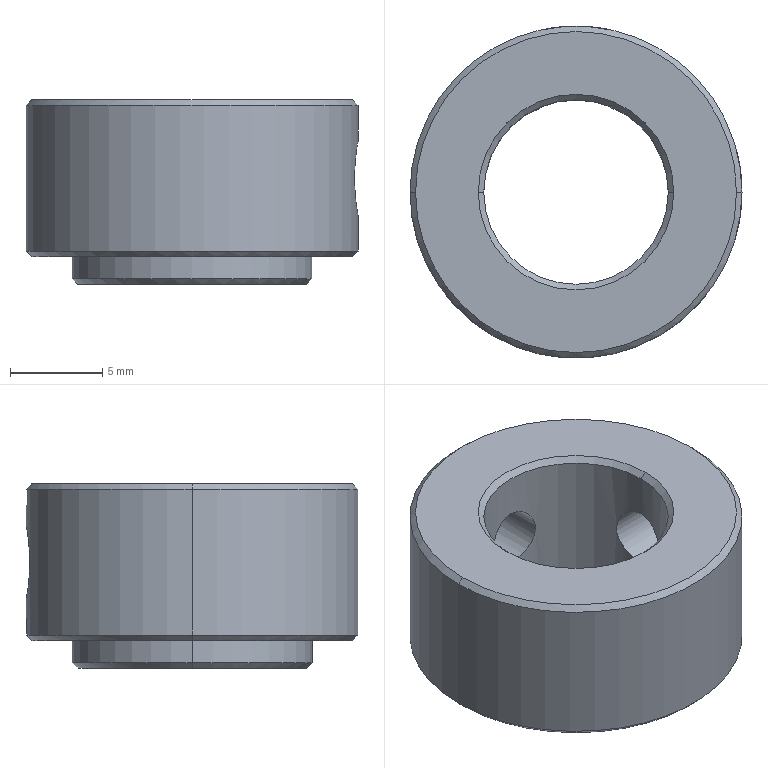Part | SolidWorks | features BaseBody 1 | 1 solid | 27 faces | box 18 x 18 x 10 mm | volume 1499 mm3 | cone 14 | cylinder 10 | plane 3 | commonest cylinder face diameters 3.242 x4 10 x2 13 x2 18 x2
STEP:
#1=CARTESIAN_POINT('',(0.,8.621,4.129));
#2=VERTEX_POINT('',#1);
#3=CARTESIAN_POINT('',(0.,9.,3.75));
#4=VERTEX_POINT('',#3);
#5=CARTESIAN_POINT('',(0.,9.003,3.747));
#6=DIRECTION('',(0.,0.7071,-0.7071));
#7=VECTOR('',#6,1000.);
#8=LINE('',#5,#7);
#9=EDGE_CURVE('',#2,#4,#8,.T.);
#10=ORIENTED_EDGE('',*,*,#9,.F.);
#11=CARTESIAN_POINT('',(0.,8.621,7.371));
#12=VERTEX_POINT('',#11);
#13=CARTESIAN_POINT('',(0.,8.621,5.75));
#14=DIRECTION('',(0.,-1.,0.));
#15=DIRECTION('',(0.,0.,1.));
#16=AXIS2_PLACEMENT_3D('',#13,#14,#15);
#17=CIRCLE('',#16,1.621);
#18=EDGE_CURVE('',#2,#12,#17,.T.);
#19=ORIENTED_EDGE('',*,*,#18,.T.);
#20=CARTESIAN_POINT('',(0.,9.,7.75));
#21=VERTEX_POINT('',#20);
#22=CARTESIAN_POINT('',(0.,9.003,7.753));
#23=DIRECTION('',(0.,0.7071,0.7071));
#24=VECTOR('',#23,1000.);
#25=LINE('',#22,#24);
#26=EDGE_CURVE('',#12,#21,#25,.T.);
#27=ORIENTED_EDGE('',*,*,#26,.T.);
#28=CARTESIAN_POINT('',(0.,9.,3.75));
#29=CARTESIAN_POINT('',(0.1256,9.,3.75));
#30=CARTESIAN_POINT('',(0.2518,8.997,3.765));
#31=CARTESIAN_POINT('',(0.4336,8.99,3.807));
#32=CARTESIAN_POINT('',(0.4933,8.987,3.825));
#33=CARTESIAN_POINT('',(0.6108,8.979,3.866));
#34=CARTESIAN_POINT('',(0.6697,8.975,3.891));
#35=CARTESIAN_POINT('',(0.8371,8.962,3.972));
#36=CARTESIAN_POINT('',(0.9418,8.951,4.036));
#37=CARTESIAN_POINT('',(1.089,8.934,4.15));
#38=CARTESIAN_POINT('',(1.136,8.928,4.19));
#39=CARTESIAN_POINT('',(1.227,8.916,4.277));
#40=CARTESIAN_POINT('',(1.272,8.91,4.324));
#41=CARTESIAN_POINT('',(1.394,8.892,4.465));
#42=CARTESIAN_POINT('',(1.466,8.88,4.566));
#43=CARTESIAN_POINT('',(1.591,8.859,4.78));
#44=CARTESIAN_POINT('',(1.644,8.849,4.895));
#45=CARTESIAN_POINT('',(1.772,8.824,5.25));
#46=CARTESIAN_POINT('',(1.815,8.815,5.495));
#47=CARTESIAN_POINT('',(1.815,8.815,5.875));
#48=CARTESIAN_POINT('',(1.805,8.817,6.));
#49=CARTESIAN_POINT('',(1.762,8.826,6.245));
#50=CARTESIAN_POINT('',(1.731,8.832,6.364));
#51=CARTESIAN_POINT('',(1.601,8.857,6.724));
#52=CARTESIAN_POINT('',(1.478,8.879,6.937));
#53=CARTESIAN_POINT('',(1.273,8.91,7.175));
#54=CARTESIAN_POINT('',(1.23,8.916,7.22));
#55=CARTESIAN_POINT('',(1.14,8.928,7.306));
#56=CARTESIAN_POINT('',(1.093,8.933,7.346));
#57=CARTESIAN_POINT('',(0.9931,8.945,7.424));
#58=CARTESIAN_POINT('',(0.9416,8.951,7.46));
#59=CARTESIAN_POINT('',(0.8357,8.961,7.525));
#60=CARTESIAN_POINT('',(0.7826,8.966,7.555));
#61=CARTESIAN_POINT('',(0.4976,8.989,7.692));
#62=CARTESIAN_POINT('',(0.2507,9.,7.75));
#63=CARTESIAN_POINT('',(0.,9.,7.75));
#64=B_SPLINE_CURVE_WITH_KNOTS('',3,(#28,#29,#30,#31,#32,#33,#34,#35,#36,#37,#38,#39,#40,#41,#42,#43,#44,#45,#46,#47,#48,#49,#50,#51,#52,#53,#54,#55,#56,#57,#58,#59,#60,#61,#62,#63),.UNSPECIFIED.,.F.,.F.,(4,2,2,2,2,2,2,2,2,2,2,2,2,2,2,2,2,4),(0.,0.0625,0.09375,0.125,0.1875,0.2187,0.25,0.3125,0.375,0.5,0.5625,0.625,0.75,0.7812,0.8125,0.8437,0.875,1.),.UNSPECIFIED.);
#65=EDGE_CURVE('',#4,#21,#64,.T.);
#66=ORIENTED_EDGE('',*,*,#65,.F.);
#67=EDGE_LOOP('',(#10,#19,#27,#66));
#68=FACE_OUTER_BOUND('',#67,.T.);
#69=CARTESIAN_POINT('',(0.,9.003,5.75));
#70=DIRECTION('',(0.,1.,0.));
#71=DIRECTION('',(0.,0.,1.));
#72=AXIS2_PLACEMENT_3D('',#69,#70,#71);
#73=CONICAL_SURFACE('',#72,2.003,0.7854);
#74=ADVANCED_FACE('',(#68),#73,.F.);
#75=CARTESIAN_POINT('',(8.621,0.,7.371));
#76=VERTEX_POINT('',#75);
#77=CARTESIAN_POINT('',(9.,0.,7.75));
#78=VERTEX_POINT('',#77);
#79=CARTESIAN_POINT('',(9.031,0.,7.781));
#80=DIRECTION('',(0.7071,0.,0.7071));
#81=VECTOR('',#80,1000.);
#82=LINE('',#79,#81);
#83=EDGE_CURVE('',#76,#78,#82,.T.);
#84=ORIENTED_EDGE('',*,*,#83,.F.);
#85=CARTESIAN_POINT('',(8.621,0.,4.129));
#86=VERTEX_POINT('',#85);
#87=CARTESIAN_POINT('',(8.621,0.,5.75));
#88=DIRECTION('',(-1.,0.,0.));
#89=DIRECTION('',(0.,0.,-1.));
#90=AXIS2_PLACEMENT_3D('',#87,#88,#89);
#91=CIRCLE('',#90,1.621);
#92=EDGE_CURVE('',#76,#86,#91,.T.);
#93=ORIENTED_EDGE('',*,*,#92,.T.);
#94=CARTESIAN_POINT('',(9.,0.,3.75));
#95=VERTEX_POINT('',#94);
#96=CARTESIAN_POINT('',(9.031,0.,3.719));
#97=DIRECTION('',(0.7071,0.,-0.7071));
#98=VECTOR('',#97,1000.);
#99=LINE('',#96,#98);
#100=EDGE_CURVE('',#86,#95,#99,.T.);
#101=ORIENTED_EDGE('',*,*,#100,.T.);
#102=CARTESIAN_POINT('',(9.,0.,7.75));
#103=CARTESIAN_POINT('',(9.,0.251,7.75));
#104=CARTESIAN_POINT('',(8.989,0.5004,7.691));
#105=CARTESIAN_POINT('',(8.962,0.8348,7.53));
#106=CARTESIAN_POINT('',(8.951,0.9395,7.465));
#107=CARTESIAN_POINT('',(8.934,1.086,7.352));
#108=CARTESIAN_POINT('',(8.928,1.133,7.312));
#109=CARTESIAN_POINT('',(8.916,1.224,7.226));
#110=CARTESIAN_POINT('',(8.91,1.27,7.178));
#111=CARTESIAN_POINT('',(8.892,1.392,7.038));
#112=CARTESIAN_POINT('',(8.88,1.464,6.937));
#113=CARTESIAN_POINT('',(8.859,1.589,6.724));
#114=CARTESIAN_POINT('',(8.849,1.642,6.609));
#115=CARTESIAN_POINT('',(8.833,1.728,6.373));
#116=CARTESIAN_POINT('',(8.826,1.76,6.253));
#117=CARTESIAN_POINT('',(8.817,1.804,6.008));
#118=CARTESIAN_POINT('',(8.815,1.815,5.883));
#119=CARTESIAN_POINT('',(8.815,1.815,5.632));
#120=CARTESIAN_POINT('',(8.817,1.805,5.506));
#121=CARTESIAN_POINT('',(8.826,1.762,5.257));
#122=CARTESIAN_POINT('',(8.832,1.731,5.136));
#123=CARTESIAN_POINT('',(8.848,1.646,4.9));
#124=CARTESIAN_POINT('',(8.858,1.594,4.788));
#125=CARTESIAN_POINT('',(8.874,1.499,4.624));
#126=CARTESIAN_POINT('',(8.88,1.466,4.571));
#127=CARTESIAN_POINT('',(8.892,1.394,4.47));
#128=CARTESIAN_POINT('',(8.897,1.356,4.422));
#129=CARTESIAN_POINT('',(8.916,1.232,4.278));
#130=CARTESIAN_POINT('',(8.928,1.144,4.193));
#131=CARTESIAN_POINT('',(8.945,0.9941,4.077));
#132=CARTESIAN_POINT('',(8.951,0.9428,4.041));
#133=CARTESIAN_POINT('',(8.961,0.837,3.975));
#134=CARTESIAN_POINT('',(8.966,0.7839,3.946));
#135=CARTESIAN_POINT('',(8.98,0.6128,3.863));
#136=CARTESIAN_POINT('',(8.987,0.4964,3.822));
#137=CARTESIAN_POINT('',(8.997,0.2502,3.764));
#138=CARTESIAN_POINT('',(9.,0.1257,3.75));
#139=CARTESIAN_POINT('',(9.,0.,3.75));
#140=B_SPLINE_CURVE_WITH_KNOTS('',3,(#102,#103,#104,#105,#106,#107,#108,#109,#110,#111,#112,#113,#114,#115,#116,#117,#118,#119,#120,#121,#122,#123,#124,#125,#126,#127,#128,#129,#130,#131,#132,#133,#134,#135,#136,#137,#138,#139),.UNSPECIFIED.,.F.,.F.,(4,2,2,2,2,2,2,2,2,2,2,2,2,2,2,2,2,2,4),(0.,0.125,0.1875,0.2187,0.25,0.3125,0.375,0.4375,0.5,0.5625,0.625,0.6875,0.7188,0.75,0.8125,0.8438,0.875,0.9375,1.),.UNSPECIFIED.);
#141=EDGE_CURVE('',#78,#95,#140,.T.);
#142=ORIENTED_EDGE('',*,*,#141,.F.);
#143=EDGE_LOOP('',(#84,#93,#101,#142));
#144=FACE_OUTER_BOUND('',#143,.T.);
#145=CARTESIAN_POINT('',(9.031,0.,5.75));
#146=DIRECTION('',(1.,0.,0.));
#147=DIRECTION('',(0.,0.,-1.));
#148=AXIS2_PLACEMENT_3D('',#145,#146,#147);
#149=CONICAL_SURFACE('',#148,2.031,0.7854);
#150=ADVANCED_FACE('',(#144),#149,.F.);
#151=CARTESIAN_POINT('',(5.,0.,0.3));
#152=VERTEX_POINT('',#151);
#153=CARTESIAN_POINT('',(5.3,0.,0.));
#154=VERTEX_POINT('',#153);
#155=CARTESIAN_POINT('',(5.3,0.,0.));
#156=DIRECTION('',(0.7071,0.,-0.7071));
#157=VECTOR('',#156,1000.);
#158=LINE('',#155,#157);
#159=EDGE_CURVE('',#152,#154,#158,.T.);
#160=ORIENTED_EDGE('',*,*,#159,.F.);
#161=CARTESIAN_POINT('',(-5.,0.,0.3));
#162=VERTEX_POINT('',#161);
#163=CARTESIAN_POINT('',(0.,0.,0.3));
#164=DIRECTION('',(0.,0.,1.));
#165=DIRECTION('',(-1.,0.,0.));
#166=AXIS2_PLACEMENT_3D('',#163,#164,#165);
#167=CIRCLE('',#166,5.);
#168=EDGE_CURVE('',#152,#162,#167,.T.);
#169=ORIENTED_EDGE('',*,*,#168,.T.);
#170=CARTESIAN_POINT('',(-5.3,0.,0.));
#171=VERTEX_POINT('',#170);
#172=CARTESIAN_POINT('',(-5.3,0.,0.));
#173=DIRECTION('',(-0.7071,0.,-0.7071));
#174=VECTOR('',#173,1000.);
#175=LINE('',#172,#174);
#176=EDGE_CURVE('',#162,#171,#175,.T.);
#177=ORIENTED_EDGE('',*,*,#176,.T.);
#178=CARTESIAN_POINT('',(0.,0.,0.));
#179=DIRECTION('',(0.,0.,1.));
#180=DIRECTION('',(-1.,0.,0.));
#181=AXIS2_PLACEMENT_3D('',#178,#179,#180);
#182=CIRCLE('',#181,5.3);
#183=EDGE_CURVE('',#154,#171,#182,.T.);
#184=ORIENTED_EDGE('',*,*,#183,.F.);
#185=EDGE_LOOP('',(#160,#169,#177,#184));
#186=FACE_OUTER_BOUND('',#185,.T.);
#187=CARTESIAN_POINT('',(0.,0.,0.));
#188=DIRECTION('',(0.,0.,-1.));
#189=DIRECTION('',(-1.,0.,0.));
#190=AXIS2_PLACEMENT_3D('',#187,#188,#189);
#191=CONICAL_SURFACE('',#190,5.3,0.7854);
#192=ADVANCED_FACE('',(#186),#191,.F.);
#193=CARTESIAN_POINT('',(0.,5.,4.129));
#194=VERTEX_POINT('',#193);
#195=CARTESIAN_POINT('',(0.,9.,4.129));
#196=DIRECTION('',(0.,1.,0.));
#197=VECTOR('',#196,1000.);
#198=LINE('',#195,#197);
#199=EDGE_CURVE('',#194,#2,#198,.T.);
#200=ORIENTED_EDGE('',*,*,#199,.F.);
#201=CARTESIAN_POINT('',(0.,5.,7.371));
#202=VERTEX_POINT('',#201);
#203=CARTESIAN_POINT('',(0.,5.,4.129));
#204=CARTESIAN_POINT('',(0.101,5.,4.129));
#205=CARTESIAN_POINT('',(0.2048,4.997,4.138));
#206=CARTESIAN_POINT('',(0.3616,4.987,4.169));
#207=CARTESIAN_POINT('',(0.414,4.983,4.182));
#208=CARTESIAN_POINT('',(0.4924,4.976,4.205));
#209=CARTESIAN_POINT('',(0.5316,4.972,4.218));
#210=CARTESIAN_POINT('',(0.577,4.967,4.235));
#211=CARTESIAN_POINT('',(0.5997,4.964,4.244));
#212=CARTESIAN_POINT('',(0.6094,4.963,4.248));
#213=CARTESIAN_POINT('',(0.6159,4.962,4.251));
#214=CARTESIAN_POINT('',(0.6202,4.961,4.252));
#215=CARTESIAN_POINT('',(0.6914,4.952,4.282));
#216=CARTESIAN_POINT('',(0.7729,4.94,4.321));
#217=CARTESIAN_POINT('',(0.9071,4.917,4.405));
#218=CARTESIAN_POINT('',(0.9537,4.908,4.438));
#219=CARTESIAN_POINT('',(1.025,4.894,4.494));
#220=CARTESIAN_POINT('',(1.049,4.889,4.514));
#221=CARTESIAN_POINT('',(1.097,4.878,4.556));
#222=CARTESIAN_POINT('',(1.12,4.873,4.578));
#223=CARTESIAN_POINT('',(1.247,4.843,4.704));
#224=CARTESIAN_POINT('',(1.321,4.823,4.805));
#225=CARTESIAN_POINT('',(1.405,4.799,4.939));
#226=CARTESIAN_POINT('',(1.428,4.792,4.982));
#227=CARTESIAN_POINT('',(1.457,4.783,5.04));
#228=CARTESIAN_POINT('',(1.466,4.78,5.059));
#229=CARTESIAN_POINT('',(1.479,4.776,5.085));
#230=CARTESIAN_POINT('',(1.484,4.775,5.098));
#231=CARTESIAN_POINT('',(1.491,4.773,5.113));
#232=CARTESIAN_POINT('',(1.493,4.772,5.119));
#233=CARTESIAN_POINT('',(1.495,4.771,5.123));
#234=CARTESIAN_POINT('',(1.495,4.771,5.124));
#235=CARTESIAN_POINT('',(1.583,4.744,5.336));
#236=CARTESIAN_POINT('',(1.621,4.73,5.551));
#237=CARTESIAN_POINT('',(1.621,4.73,5.851));
#238=CARTESIAN_POINT('',(1.612,4.733,5.954));
#239=CARTESIAN_POINT('',(1.581,4.744,6.111));
#240=CARTESIAN_POINT('',(1.568,4.748,6.163));
#241=CARTESIAN_POINT('',(1.545,4.755,6.242));
#242=CARTESIAN_POINT('',(1.532,4.76,6.282));
#243=CARTESIAN_POINT('',(1.515,4.765,6.327));
#244=CARTESIAN_POINT('',(1.506,4.768,6.35));
#245=CARTESIAN_POINT('',(1.502,4.769,6.36));
#246=CARTESIAN_POINT('',(1.499,4.77,6.367));
#247=CARTESIAN_POINT('',(1.497,4.771,6.371));
#248=CARTESIAN_POINT('',(1.47,4.779,6.437));
#249=CARTESIAN_POINT('',(1.433,4.791,6.516));
#250=CARTESIAN_POINT('',(1.349,4.815,6.65));
#251=CARTESIAN_POINT('',(1.317,4.824,6.697));
#252=CARTESIAN_POINT('',(1.26,4.839,6.771));
#253=CARTESIAN_POINT('',(1.239,4.844,6.796));
#254=CARTESIAN_POINT('',(1.195,4.855,6.846));
#255=CARTESIAN_POINT('',(1.171,4.861,6.872));
#256=CARTESIAN_POINT('',(1.05,4.89,6.993));
#257=CARTESIAN_POINT('',(0.9525,4.909,7.066));
#258=CARTESIAN_POINT('',(0.8184,4.932,7.15));
#259=CARTESIAN_POINT('',(0.7756,4.939,7.174));
#260=CARTESIAN_POINT('',(0.7153,4.948,7.205));
#261=CARTESIAN_POINT('',(0.6862,4.953,7.219));
#262=CARTESIAN_POINT('',(0.654,4.957,7.233));
#263=CARTESIAN_POINT('',(0.6385,4.959,7.24));
#264=CARTESIAN_POINT('',(0.6319,4.96,7.243));
#265=CARTESIAN_POINT('',(0.6275,4.96,7.245));
#266=CARTESIAN_POINT('',(0.6264,4.961,7.245));
#267=CARTESIAN_POINT('',(0.4163,4.987,7.333));
#268=CARTESIAN_POINT('',(0.2023,5.,7.371));
#269=CARTESIAN_POINT('',(0.,5.,7.371));
#270=B_SPLINE_CURVE_WITH_KNOTS('',3,(#203,#204,#205,#206,#207,#208,#209,#210,#211,#212,#213,#214,#215,#216,#217,#218,#219,#220,#221,#222,#223,#224,#225,#226,#227,#228,#229,#230,#231,#232,#233,#234,#235,#236,#237,#238,#239,#240,#241,#242,#243,#244,#245,#246,#247,#248,#249,#250,#251,#252,#253,#254,#255,#256,#257,#258,#259,#260,#261,#262,#263,#264,#265,#266,#267,#268,#269),.UNSPECIFIED.,.F.,.F.,(4,2,2,1,1,1,2,2,2,2,2,2,2,2,2,1,1,2,2,2,2,2,1,1,1,2,2,2,2,2,2,2,2,1,1,1,2,2,4),(0.,0.0625,0.09375,0.1094,0.1172,0.1211,0.123,0.125,0.1875,0.2187,0.2344,0.25,0.3125,0.3437,0.3594,0.3672,0.3711,0.373,0.375,0.5,0.5625,0.5938,0.6094,0.6172,0.6211,0.623,0.625,0.6875,0.7188,0.7344,0.75,0.8125,0.8438,0.8594,0.8672,0.8711,0.873,0.875,1.),.UNSPECIFIED.);
#271=EDGE_CURVE('',#194,#202,#270,.T.);
#272=ORIENTED_EDGE('',*,*,#271,.T.);
#273=CARTESIAN_POINT('',(0.,9.,7.371));
#274=DIRECTION('',(0.,1.,0.));
#275=VECTOR('',#274,1000.);
#276=LINE('',#273,#275);
#277=EDGE_CURVE('',#202,#12,#276,.T.);
#278=ORIENTED_EDGE('',*,*,#277,.T.);
#279=ORIENTED_EDGE('',*,*,#18,.F.);
#280=EDGE_LOOP('',(#200,#272,#278,#279));
#281=FACE_OUTER_BOUND('',#280,.T.);
#282=CARTESIAN_POINT('',(0.,9.,5.75));
#283=DIRECTION('',(0.,1.,0.));
#284=DIRECTION('',(0.,0.,1.));
#285=AXIS2_PLACEMENT_3D('',#282,#283,#284);
#286=CYLINDRICAL_SURFACE('',#285,1.621);
#287=ADVANCED_FACE('',(#281),#286,.F.);
#288=CARTESIAN_POINT('',(5.,0.,4.129));
#289=VERTEX_POINT('',#288);
#290=CARTESIAN_POINT('',(0.,0.,4.129));
#291=DIRECTION('',(-1.,0.,0.));
#292=VECTOR('',#291,1000.);
#293=LINE('',#290,#292);
#294=EDGE_CURVE('',#86,#289,#293,.T.);
#295=ORIENTED_EDGE('',*,*,#294,.F.);
#296=ORIENTED_EDGE('',*,*,#92,.F.);
#297=CARTESIAN_POINT('',(5.,0.,7.371));
#298=VERTEX_POINT('',#297);
#299=CARTESIAN_POINT('',(0.,0.,7.371));
#300=DIRECTION('',(-1.,0.,0.));
#301=VECTOR('',#300,1000.);
#302=LINE('',#299,#301);
#303=EDGE_CURVE('',#76,#298,#302,.T.);
#304=ORIENTED_EDGE('',*,*,#303,.T.);
#305=CARTESIAN_POINT('',(5.,0.,7.371));
#306=CARTESIAN_POINT('',(5.,0.1011,7.371));
#307=CARTESIAN_POINT('',(4.997,0.205,7.362));
#308=CARTESIAN_POINT('',(4.987,0.362,7.331));
#309=CARTESIAN_POINT('',(4.983,0.4145,7.318));
#310=CARTESIAN_POINT('',(4.976,0.493,7.294));
#311=CARTESIAN_POINT('',(4.972,0.5322,7.282));
#312=CARTESIAN_POINT('',(4.967,0.5778,7.265));
#313=CARTESIAN_POINT('',(4.964,0.6005,7.256));
#314=CARTESIAN_POINT('',(4.963,0.6102,7.252));
#315=CARTESIAN_POINT('',(4.962,0.6167,7.249));
#316=CARTESIAN_POINT('',(4.961,0.621,7.247));
#317=CARTESIAN_POINT('',(4.952,0.6921,7.218));
#318=CARTESIAN_POINT('',(4.94,0.7736,7.178));
#319=CARTESIAN_POINT('',(4.917,0.9077,7.094));
#320=CARTESIAN_POINT('',(4.908,0.9543,7.062));
#321=CARTESIAN_POINT('',(4.893,1.026,7.006));
#322=CARTESIAN_POINT('',(4.888,1.05,6.986));
#323=CARTESIAN_POINT('',(4.881,1.086,6.954));
#324=CARTESIAN_POINT('',(4.878,1.098,6.943));
#325=CARTESIAN_POINT('',(4.872,1.122,6.92));
#326=CARTESIAN_POINT('',(4.87,1.133,6.909));
#327=CARTESIAN_POINT('',(4.855,1.198,6.845));
#328=CARTESIAN_POINT('',(4.844,1.239,6.797));
#329=CARTESIAN_POINT('',(4.831,1.288,6.735));
#330=CARTESIAN_POINT('',(4.828,1.302,6.716));
#331=CARTESIAN_POINT('',(4.822,1.321,6.69));
#332=CARTESIAN_POINT('',(4.82,1.329,6.678));
#333=CARTESIAN_POINT('',(4.818,1.338,6.665));
#334=CARTESIAN_POINT('',(4.817,1.342,6.66));
#335=CARTESIAN_POINT('',(4.816,1.344,6.656));
#336=CARTESIAN_POINT('',(4.816,1.344,6.656));
#337=CARTESIAN_POINT('',(4.806,1.379,6.604));
#338=CARTESIAN_POINT('',(4.798,1.408,6.556));
#339=CARTESIAN_POINT('',(4.787,1.445,6.486));
#340=CARTESIAN_POINT('',(4.782,1.462,6.451));
#341=CARTESIAN_POINT('',(4.776,1.48,6.412));
#342=CARTESIAN_POINT('',(4.774,1.487,6.395));
#343=CARTESIAN_POINT('',(4.772,1.492,6.384));
#344=CARTESIAN_POINT('',(4.772,1.494,6.379));
#345=CARTESIAN_POINT('',(4.744,1.583,6.165));
#346=CARTESIAN_POINT('',(4.73,1.621,5.951));
#347=CARTESIAN_POINT('',(4.73,1.621,5.65));
#348=CARTESIAN_POINT('',(4.733,1.612,5.547));
#349=CARTESIAN_POINT('',(4.743,1.581,5.39));
#350=CARTESIAN_POINT('',(4.748,1.569,5.338));
#351=CARTESIAN_POINT('',(4.755,1.545,5.259));
#352=CARTESIAN_POINT('',(4.76,1.532,5.22));
#353=CARTESIAN_POINT('',(4.765,1.515,5.174));
#354=CARTESIAN_POINT('',(4.767,1.508,5.154));
#355=CARTESIAN_POINT('',(4.769,1.502,5.141));
#356=CARTESIAN_POINT('',(4.77,1.499,5.134));
#357=CARTESIAN_POINT('',(4.776,1.479,5.084));
#358=CARTESIAN_POINT('',(4.783,1.458,5.039));
#359=CARTESIAN_POINT('',(4.794,1.421,4.969));
#360=CARTESIAN_POINT('',(4.8,1.401,4.933));
#361=CARTESIAN_POINT('',(4.807,1.375,4.891));
#362=CARTESIAN_POINT('',(4.811,1.361,4.87));
#363=CARTESIAN_POINT('',(4.813,1.355,4.861));
#364=CARTESIAN_POINT('',(4.814,1.351,4.854));
#365=CARTESIAN_POINT('',(4.815,1.348,4.85));
#366=CARTESIAN_POINT('',(4.82,1.329,4.821));
#367=CARTESIAN_POINT('',(4.827,1.305,4.787));
#368=CARTESIAN_POINT('',(4.84,1.256,4.725));
#369=CARTESIAN_POINT('',(4.845,1.237,4.702));
#370=CARTESIAN_POINT('',(4.852,1.206,4.667));
#371=CARTESIAN_POINT('',(4.855,1.195,4.655));
#372=CARTESIAN_POINT('',(4.861,1.172,4.63));
#373=CARTESIAN_POINT('',(4.864,1.159,4.617));
#374=CARTESIAN_POINT('',(4.889,1.05,4.508));
#375=CARTESIAN_POINT('',(4.909,0.9526,4.434));
#376=CARTESIAN_POINT('',(4.932,0.8183,4.35));
#377=CARTESIAN_POINT('',(4.939,0.7755,4.326));
#378=CARTESIAN_POINT('',(4.948,0.7151,4.295));
#379=CARTESIAN_POINT('',(4.953,0.6859,4.281));
#380=CARTESIAN_POINT('',(4.957,0.6538,4.267));
#381=CARTESIAN_POINT('',(4.959,0.6382,4.26));
#382=CARTESIAN_POINT('',(4.96,0.6316,4.257));
#383=CARTESIAN_POINT('',(4.96,0.6272,4.255));
#384=CARTESIAN_POINT('',(4.961,0.6262,4.255));
#385=CARTESIAN_POINT('',(4.987,0.4161,4.167));
#386=CARTESIAN_POINT('',(5.,0.2022,4.129));
#387=CARTESIAN_POINT('',(5.,0.,4.129));
#388=B_SPLINE_CURVE_WITH_KNOTS('',3,(#305,#306,#307,#308,#309,#310,#311,#312,#313,#314,#315,#316,#317,#318,#319,#320,#321,#322,#323,#324,#325,#326,#327,#328,#329,#330,#331,#332,#333,#334,#335,#336,#337,#338,#339,#340,#341,#342,#343,#344,#345,#346,#347,#348,#349,#350,#351,#352,#353,#354,#355,#356,#357,#358,#359,#360,#361,#362,#363,#364,#365,#366,#367,#368,#369,#370,#371,#372,#373,#374,#375,#376,#377,#378,#379,#380,#381,#382,#383,#384,#385,#386,#387),.UNSPECIFIED.,.F.,.F.,(4,2,2,1,1,1,2,2,2,2,2,2,2,2,2,1,1,2,2,2,1,1,2,2,2,2,2,1,1,2,2,2,1,1,1,2,2,2,2,2,2,2,2,1,1,1,2,2,4),(0.,0.0625,0.09375,0.1094,0.1172,0.1211,0.123,0.125,0.1875,0.2188,0.2344,0.2422,0.25,0.2813,0.2969,0.3047,0.3086,0.3105,0.3125,0.3438,0.3594,0.3672,0.3711,0.375,0.5,0.5625,0.5938,0.6094,0.6172,0.6211,0.625,0.6563,0.6719,0.6797,0.6836,0.6855,0.6875,0.7188,0.7344,0.7422,0.75,0.8125,0.8438,0.8594,0.8672,0.8711,0.873,0.875,1.),.UNSPECIFIED.);
#389=EDGE_CURVE('',#298,#289,#388,.T.);
#390=ORIENTED_EDGE('',*,*,#389,.T.);
#391=EDGE_LOOP('',(#295,#296,#304,#390));
#392=FACE_OUTER_BOUND('',#391,.T.);
#393=CARTESIAN_POINT('',(0.,0.,5.75));
#394=DIRECTION('',(-1.,0.,0.));
#395=DIRECTION('',(0.,0.,1.));
#396=AXIS2_PLACEMENT_3D('',#393,#394,#395);
#397=CYLINDRICAL_SURFACE('',#396,1.621);
#398=ADVANCED_FACE('',(#392),#397,.F.);
#399=CARTESIAN_POINT('',(0.,0.,0.));
#400=DIRECTION('',(0.,0.,1.));
#401=DIRECTION('',(-1.,0.,0.));
#402=AXIS2_PLACEMENT_3D('',#399,#400,#401);
#403=CIRCLE('',#402,5.3);
#404=EDGE_CURVE('',#171,#154,#403,.T.);
#405=ORIENTED_EDGE('',*,*,#404,.T.);
#406=ORIENTED_EDGE('',*,*,#183,.T.);
#407=EDGE_LOOP('',(#405,#406));
#408=FACE_BOUND('',#407,.T.);
#409=CARTESIAN_POINT('',(6.2,0.,0.));
#410=VERTEX_POINT('',#409);
#411=CARTESIAN_POINT('',(-6.2,0.,0.));
#412=VERTEX_POINT('',#411);
#413=CARTESIAN_POINT('',(0.,0.,0.));
#414=DIRECTION('',(0.,0.,1.));
#415=DIRECTION('',(1.,0.,0.));
#416=AXIS2_PLACEMENT_3D('',#413,#414,#415);
#417=CIRCLE('',#416,6.2);
#418=EDGE_CURVE('',#410,#412,#417,.T.);
#419=ORIENTED_EDGE('',*,*,#418,.F.);
#420=CARTESIAN_POINT('',(0.,0.,0.));
#421=DIRECTION('',(0.,0.,1.));
#422=DIRECTION('',(1.,0.,0.));
#423=AXIS2_PLACEMENT_3D('',#420,#421,#422);
#424=CIRCLE('',#423,6.2);
#425=EDGE_CURVE('',#412,#410,#424,.T.);
#426=ORIENTED_EDGE('',*,*,#425,.F.);
#427=EDGE_LOOP('',(#419,#426));
#428=FACE_OUTER_BOUND('',#427,.T.);
#429=CARTESIAN_POINT('',(0.,5.3,0.));
#430=DIRECTION('',(0.,0.,-1.));
#431=DIRECTION('',(0.,-1.,0.));
#432=AXIS2_PLACEMENT_3D('',#429,#430,#431);
#433=PLANE('',#432);
#434=ADVANCED_FACE('',(#408,#428),#433,.T.);
#435=CARTESIAN_POINT('',(0.,5.,7.371));
#436=CARTESIAN_POINT('',(-0.1011,5.,7.371));
#437=CARTESIAN_POINT('',(-0.205,4.997,7.362));
#438=CARTESIAN_POINT('',(-0.362,4.987,7.331));
#439=CARTESIAN_POINT('',(-0.4145,4.983,7.318));
#440=CARTESIAN_POINT('',(-0.493,4.976,7.294));
#441=CARTESIAN_POINT('',(-0.5322,4.972,7.282));
#442=CARTESIAN_POINT('',(-0.5778,4.967,7.265));
#443=CARTESIAN_POINT('',(-0.6005,4.964,7.256));
#444=CARTESIAN_POINT('',(-0.6102,4.963,7.252));
#445=CARTESIAN_POINT('',(-0.6167,4.962,7.249));
#446=CARTESIAN_POINT('',(-0.621,4.961,7.247));
#447=CARTESIAN_POINT('',(-0.6921,4.952,7.218));
#448=CARTESIAN_POINT('',(-0.7736,4.94,7.178));
#449=CARTESIAN_POINT('',(-0.9077,4.917,7.094));
#450=CARTESIAN_POINT('',(-0.9543,4.908,7.062));
#451=CARTESIAN_POINT('',(-1.026,4.893,7.006));
#452=CARTESIAN_POINT('',(-1.05,4.888,6.986));
#453=CARTESIAN_POINT('',(-1.086,4.881,6.954));
#454=CARTESIAN_POINT('',(-1.098,4.878,6.943));
#455=CARTESIAN_POINT('',(-1.122,4.872,6.92));
#456=CARTESIAN_POINT('',(-1.133,4.87,6.909));
#457=CARTESIAN_POINT('',(-1.198,4.855,6.845));
#458=CARTESIAN_POINT('',(-1.239,4.844,6.797));
#459=CARTESIAN_POINT('',(-1.288,4.831,6.735));
#460=CARTESIAN_POINT('',(-1.302,4.828,6.716));
#461=CARTESIAN_POINT('',(-1.321,4.822,6.69));
#462=CARTESIAN_POINT('',(-1.329,4.82,6.678));
#463=CARTESIAN_POINT('',(-1.338,4.818,6.665));
#464=CARTESIAN_POINT('',(-1.342,4.817,6.66));
#465=CARTESIAN_POINT('',(-1.344,4.816,6.656));
#466=CARTESIAN_POINT('',(-1.344,4.816,6.656));
#467=CARTESIAN_POINT('',(-1.379,4.806,6.604));
#468=CARTESIAN_POINT('',(-1.408,4.798,6.556));
#469=CARTESIAN_POINT('',(-1.445,4.787,6.486));
#470=CARTESIAN_POINT('',(-1.462,4.782,6.451));
#471=CARTESIAN_POINT('',(-1.48,4.776,6.412));
#472=CARTESIAN_POINT('',(-1.487,4.774,6.395));
#473=CARTESIAN_POINT('',(-1.492,4.772,6.384));
#474=CARTESIAN_POINT('',(-1.494,4.772,6.379));
#475=CARTESIAN_POINT('',(-1.583,4.744,6.165));
#476=CARTESIAN_POINT('',(-1.621,4.73,5.951));
#477=CARTESIAN_POINT('',(-1.621,4.73,5.65));
#478=CARTESIAN_POINT('',(-1.612,4.733,5.547));
#479=CARTESIAN_POINT('',(-1.581,4.743,5.39));
#480=CARTESIAN_POINT('',(-1.569,4.748,5.338));
#481=CARTESIAN_POINT('',(-1.545,4.755,5.259));
#482=CARTESIAN_POINT('',(-1.532,4.76,5.22));
#483=CARTESIAN_POINT('',(-1.515,4.765,5.174));
#484=CARTESIAN_POINT('',(-1.508,4.767,5.154));
#485=CARTESIAN_POINT('',(-1.502,4.769,5.141));
#486=CARTESIAN_POINT('',(-1.499,4.77,5.134));
#487=CARTESIAN_POINT('',(-1.479,4.776,5.084));
#488=CARTESIAN_POINT('',(-1.458,4.783,5.039));
#489=CARTESIAN_POINT('',(-1.421,4.794,4.969));
#490=CARTESIAN_POINT('',(-1.401,4.8,4.933));
#491=CARTESIAN_POINT('',(-1.375,4.807,4.891));
#492=CARTESIAN_POINT('',(-1.361,4.811,4.87));
#493=CARTESIAN_POINT('',(-1.355,4.813,4.861));
#494=CARTESIAN_POINT('',(-1.351,4.814,4.854));
#495=CARTESIAN_POINT('',(-1.348,4.815,4.85));
#496=CARTESIAN_POINT('',(-1.329,4.82,4.821));
#497=CARTESIAN_POINT('',(-1.305,4.827,4.787));
#498=CARTESIAN_POINT('',(-1.256,4.84,4.725));
#499=CARTESIAN_POINT('',(-1.237,4.845,4.702));
#500=CARTESIAN_POINT('',(-1.206,4.852,4.667));
#501=CARTESIAN_POINT('',(-1.195,4.855,4.655));
#502=CARTESIAN_POINT('',(-1.172,4.861,4.63));
#503=CARTESIAN_POINT('',(-1.159,4.864,4.617));
#504=CARTESIAN_POINT('',(-1.05,4.889,4.508));
#505=CARTESIAN_POINT('',(-0.9526,4.909,4.434));
#506=CARTESIAN_POINT('',(-0.8183,4.932,4.35));
#507=CARTESIAN_POINT('',(-0.7755,4.939,4.326));
#508=CARTESIAN_POINT('',(-0.7151,4.948,4.295));
#509=CARTESIAN_POINT('',(-0.6859,4.953,4.281));
#510=CARTESIAN_POINT('',(-0.6538,4.957,4.267));
#511=CARTESIAN_POINT('',(-0.6382,4.959,4.26));
#512=CARTESIAN_POINT('',(-0.6316,4.96,4.257));
#513=CARTESIAN_POINT('',(-0.6272,4.96,4.255));
#514=CARTESIAN_POINT('',(-0.6262,4.961,4.255));
#515=CARTESIAN_POINT('',(-0.4161,4.987,4.167));
#516=CARTESIAN_POINT('',(-0.2022,5.,4.129));
#517=CARTESIAN_POINT('',(0.,5.,4.129));
#518=B_SPLINE_CURVE_WITH_KNOTS('',3,(#435,#436,#437,#438,#439,#440,#441,#442,#443,#444,#445,#446,#447,#448,#449,#450,#451,#452,#453,#454,#455,#456,#457,#458,#459,#460,#461,#462,#463,#464,#465,#466,#467,#468,#469,#470,#471,#472,#473,#474,#475,#476,#477,#478,#479,#480,#481,#482,#483,#484,#485,#486,#487,#488,#489,#490,#491,#492,#493,#494,#495,#496,#497,#498,#499,#500,#501,#502,#503,#504,#505,#506,#507,#508,#509,#510,#511,#512,#513,#514,#515,#516,#517),.UNSPECIFIED.,.F.,.F.,(4,2,2,1,1,1,2,2,2,2,2,2,2,2,2,1,1,2,2,2,1,1,2,2,2,2,2,1,1,2,2,2,1,1,1,2,2,2,2,2,2,2,2,1,1,1,2,2,4),(0.,0.0625,0.09375,0.1094,0.1172,0.1211,0.123,0.125,0.1875,0.2188,0.2344,0.2422,0.25,0.2813,0.2969,0.3047,0.3086,0.3105,0.3125,0.3438,0.3594,0.3672,0.3711,0.375,0.5,0.5625,0.5938,0.6094,0.6172,0.6211,0.625,0.6563,0.6719,0.6797,0.6836,0.6855,0.6875,0.7188,0.7344,0.7422,0.75,0.8125,0.8438,0.8594,0.8672,0.8711,0.873,0.875,1.),.UNSPECIFIED.);
#519=EDGE_CURVE('',#202,#194,#518,.T.);
#520=ORIENTED_EDGE('',*,*,#519,.F.);
#521=ORIENTED_EDGE('',*,*,#271,.F.);
#522=EDGE_LOOP('',(#520,#521));
#523=FACE_BOUND('',#522,.T.);
#524=CARTESIAN_POINT('',(5.,0.,9.7));
#525=VERTEX_POINT('',#524);
#526=CARTESIAN_POINT('',(5.,0.,0.));
#527=DIRECTION('',(0.,0.,-1.));
#528=VECTOR('',#527,1000.);
#529=LINE('',#526,#528);
#530=EDGE_CURVE('',#525,#298,#529,.T.);
#531=ORIENTED_EDGE('',*,*,#530,.F.);
#532=CARTESIAN_POINT('',(-5.,0.,9.7));
#533=VERTEX_POINT('',#532);
#534=CARTESIAN_POINT('',(0.,0.,9.7));
#535=DIRECTION('',(0.,0.,1.));
#536=DIRECTION('',(-1.,0.,0.));
#537=AXIS2_PLACEMENT_3D('',#534,#535,#536);
#538=CIRCLE('',#537,5.);
#539=EDGE_CURVE('',#525,#533,#538,.T.);
#540=ORIENTED_EDGE('',*,*,#539,.T.);
#541=CARTESIAN_POINT('',(-5.,0.,0.));
#542=DIRECTION('',(0.,0.,-1.));
#543=VECTOR('',#542,1000.);
#544=LINE('',#541,#543);
#545=EDGE_CURVE('',#533,#162,#544,.T.);
#546=ORIENTED_EDGE('',*,*,#545,.T.);
#547=ORIENTED_EDGE('',*,*,#168,.F.);
#548=CARTESIAN_POINT('',(5.,0.,0.));
#549=DIRECTION('',(0.,0.,-1.));
#550=VECTOR('',#549,1000.);
#551=LINE('',#548,#550);
#552=EDGE_CURVE('',#289,#152,#551,.T.);
#553=ORIENTED_EDGE('',*,*,#552,.F.);
#554=ORIENTED_EDGE('',*,*,#389,.F.);
#555=EDGE_LOOP('',(#531,#540,#546,#547,#553,#554));
#556=FACE_OUTER_BOUND('',#555,.T.);
#557=CARTESIAN_POINT('',(0.,0.,0.));
#558=DIRECTION('',(0.,0.,-1.));
#559=DIRECTION('',(-1.,0.,0.));
#560=AXIS2_PLACEMENT_3D('',#557,#558,#559);
#561=CYLINDRICAL_SURFACE('',#560,5.);
#562=ADVANCED_FACE('',(#523,#556),#561,.F.);
#563=CARTESIAN_POINT('',(-6.5,0.,0.3));
#564=VERTEX_POINT('',#563);
#565=CARTESIAN_POINT('',(-6.5,0.,0.3));
#566=DIRECTION('',(-0.7071,0.,0.7071));
#567=VECTOR('',#566,1000.);
#568=LINE('',#565,#567);
#569=EDGE_CURVE('',#412,#564,#568,.T.);
#570=ORIENTED_EDGE('',*,*,#569,.F.);
#571=ORIENTED_EDGE('',*,*,#425,.T.);
#572=CARTESIAN_POINT('',(6.5,0.,0.3));
#573=VERTEX_POINT('',#572);
#574=CARTESIAN_POINT('',(6.5,0.,0.3));
#575=DIRECTION('',(0.7071,0.,0.7071));
#576=VECTOR('',#575,1000.);
#577=LINE('',#574,#576);
#578=EDGE_CURVE('',#410,#573,#577,.T.);
#579=ORIENTED_EDGE('',*,*,#578,.T.);
#580=CARTESIAN_POINT('',(0.,0.,0.3));
#581=DIRECTION('',(0.,0.,1.));
#582=DIRECTION('',(-1.,0.,0.));
#583=AXIS2_PLACEMENT_3D('',#580,#581,#582);
#584=CIRCLE('',#583,6.5);
#585=EDGE_CURVE('',#564,#573,#584,.T.);
#586=ORIENTED_EDGE('',*,*,#585,.F.);
#587=EDGE_LOOP('',(#570,#571,#579,#586));
#588=FACE_OUTER_BOUND('',#587,.T.);
#589=CARTESIAN_POINT('',(0.,0.,0.3));
#590=DIRECTION('',(0.,0.,1.));
#591=DIRECTION('',(1.,0.,0.));
#592=AXIS2_PLACEMENT_3D('',#589,#590,#591);
#593=CONICAL_SURFACE('',#592,6.5,0.7854);
#594=ADVANCED_FACE('',(#588),#593,.T.);
#595=CARTESIAN_POINT('',(-5.3,0.,10.));
#596=VERTEX_POINT('',#595);
#597=CARTESIAN_POINT('',(-5.3,0.,10.));
#598=DIRECTION('',(-0.7071,0.,0.7071));
#599=VECTOR('',#598,1000.);
#600=LINE('',#597,#599);
#601=EDGE_CURVE('',#533,#596,#600,.T.);
#602=ORIENTED_EDGE('',*,*,#601,.F.);
#603=ORIENTED_EDGE('',*,*,#539,.F.);
#604=CARTESIAN_POINT('',(5.3,0.,10.));
#605=VERTEX_POINT('',#604);
#606=CARTESIAN_POINT('',(5.3,0.,10.));
#607=DIRECTION('',(0.7071,0.,0.7071));
#608=VECTOR('',#607,1000.);
#609=LINE('',#606,#608);
#610=EDGE_CURVE('',#525,#605,#609,.T.);
#611=ORIENTED_EDGE('',*,*,#610,.T.);
#612=CARTESIAN_POINT('',(0.,0.,10.));
#613=DIRECTION('',(0.,0.,-1.));
#614=DIRECTION('',(1.,0.,0.));
#615=AXIS2_PLACEMENT_3D('',#612,#613,#614);
#616=CIRCLE('',#615,5.3);
#617=EDGE_CURVE('',#596,#605,#616,.T.);
#618=ORIENTED_EDGE('',*,*,#617,.F.);
#619=EDGE_LOOP('',(#602,#603,#611,#618));
#620=FACE_OUTER_BOUND('',#619,.T.);
#621=CARTESIAN_POINT('',(0.,0.,10.));
#622=DIRECTION('',(0.,0.,1.));
#623=DIRECTION('',(1.,0.,0.));
#624=AXIS2_PLACEMENT_3D('',#621,#622,#623);
#625=CONICAL_SURFACE('',#624,5.3,0.7854);
#626=ADVANCED_FACE('',(#620),#625,.F.);
#627=CARTESIAN_POINT('',(6.5,0.,1.5));
#628=VERTEX_POINT('',#627);
#629=CARTESIAN_POINT('',(6.5,0.,0.));
#630=DIRECTION('',(0.,0.,-1.));
#631=VECTOR('',#630,1000.);
#632=LINE('',#629,#631);
#633=EDGE_CURVE('',#628,#573,#632,.T.);
#634=ORIENTED_EDGE('',*,*,#633,.F.);
#635=CARTESIAN_POINT('',(-6.5,0.,1.5));
#636=VERTEX_POINT('',#635);
#637=CARTESIAN_POINT('',(0.,0.,1.5));
#638=DIRECTION('',(0.,0.,1.));
#639=DIRECTION('',(-1.,0.,0.));
#640=AXIS2_PLACEMENT_3D('',#637,#638,#639);
#641=CIRCLE('',#640,6.5);
#642=EDGE_CURVE('',#636,#628,#641,.T.);
#643=ORIENTED_EDGE('',*,*,#642,.F.);
#644=CARTESIAN_POINT('',(-6.5,0.,0.));
#645=DIRECTION('',(0.,0.,-1.));
#646=VECTOR('',#645,1000.);
#647=LINE('',#644,#646);
#648=EDGE_CURVE('',#636,#564,#647,.T.);
#649=ORIENTED_EDGE('',*,*,#648,.T.);
#650=ORIENTED_EDGE('',*,*,#585,.T.);
#651=EDGE_LOOP('',(#634,#643,#649,#650));
#652=FACE_OUTER_BOUND('',#651,.T.);
#653=CARTESIAN_POINT('',(0.,0.,0.));
#654=DIRECTION('',(0.,0.,-1.));
#655=DIRECTION('',(-1.,0.,0.));
#656=AXIS2_PLACEMENT_3D('',#653,#654,#655);
#657=CYLINDRICAL_SURFACE('',#656,6.5);
#658=ADVANCED_FACE('',(#652),#657,.T.);
#659=CARTESIAN_POINT('',(0.,0.,10.));
#660=DIRECTION('',(0.,0.,-1.));
#661=DIRECTION('',(1.,0.,0.));
#662=AXIS2_PLACEMENT_3D('',#659,#660,#661);
#663=CIRCLE('',#662,5.3);
#664=EDGE_CURVE('',#605,#596,#663,.T.);
#665=ORIENTED_EDGE('',*,*,#664,.T.);
#666=ORIENTED_EDGE('',*,*,#617,.T.);
#667=EDGE_LOOP('',(#665,#666));
#668=FACE_BOUND('',#667,.T.);
#669=CARTESIAN_POINT('',(-8.7,0.,10.));
#670=VERTEX_POINT('',#669);
#671=CARTESIAN_POINT('',(8.7,0.,10.));
#672=VERTEX_POINT('',#671);
#673=CARTESIAN_POINT('',(0.,0.,10.));
#674=DIRECTION('',(0.,0.,-1.));
#675=DIRECTION('',(-1.,0.,0.));
#676=AXIS2_PLACEMENT_3D('',#673,#674,#675);
#677=CIRCLE('',#676,8.7);
#678=EDGE_CURVE('',#670,#672,#677,.T.);
#679=ORIENTED_EDGE('',*,*,#678,.F.);
#680=CARTESIAN_POINT('',(0.,0.,10.));
#681=DIRECTION('',(0.,0.,-1.));
#682=DIRECTION('',(-1.,0.,0.));
#683=AXIS2_PLACEMENT_3D('',#680,#681,#682);
#684=CIRCLE('',#683,8.7);
#685=EDGE_CURVE('',#672,#670,#684,.T.);
#686=ORIENTED_EDGE('',*,*,#685,.F.);
#687=EDGE_LOOP('',(#679,#686));
#688=FACE_OUTER_BOUND('',#687,.T.);
#689=CARTESIAN_POINT('',(0.,8.7,10.));
#690=DIRECTION('',(0.,0.,1.));
#691=DIRECTION('',(1.,0.,0.));
#692=AXIS2_PLACEMENT_3D('',#689,#690,#691);
#693=PLANE('',#692);
#694=ADVANCED_FACE('',(#668,#688),#693,.T.);
#695=ORIENTED_EDGE('',*,*,#642,.T.);
#696=CARTESIAN_POINT('',(0.,0.,1.5));
#697=DIRECTION('',(0.,0.,1.));
#698=DIRECTION('',(-1.,0.,0.));
#699=AXIS2_PLACEMENT_3D('',#696,#697,#698);
#700=CIRCLE('',#699,6.5);
#701=EDGE_CURVE('',#628,#636,#700,.T.);
#702=ORIENTED_EDGE('',*,*,#701,.T.);
#703=EDGE_LOOP('',(#695,#702));
#704=FACE_BOUND('',#703,.T.);
#705=CARTESIAN_POINT('',(8.7,0.,1.5));
#706=VERTEX_POINT('',#705);
#707=CARTESIAN_POINT('',(-8.7,0.,1.5));
#708=VERTEX_POINT('',#707);
#709=CARTESIAN_POINT('',(0.,0.,1.5));
#710=DIRECTION('',(0.,0.,1.));
#711=DIRECTION('',(1.,0.,0.));
#712=AXIS2_PLACEMENT_3D('',#709,#710,#711);
#713=CIRCLE('',#712,8.7);
#714=EDGE_CURVE('',#706,#708,#713,.T.);
#715=ORIENTED_EDGE('',*,*,#714,.F.);
#716=CARTESIAN_POINT('',(0.,0.,1.5));
#717=DIRECTION('',(0.,0.,1.));
#718=DIRECTION('',(1.,0.,0.));
#719=AXIS2_PLACEMENT_3D('',#716,#717,#718);
#720=CIRCLE('',#719,8.7);
#721=EDGE_CURVE('',#708,#706,#720,.T.);
#722=ORIENTED_EDGE('',*,*,#721,.F.);
#723=EDGE_LOOP('',(#715,#722));
#724=FACE_OUTER_BOUND('',#723,.T.);
#725=CARTESIAN_POINT('',(0.,6.5,1.5));
#726=DIRECTION('',(0.,0.,-1.));
#727=DIRECTION('',(0.,-1.,0.));
#728=AXIS2_PLACEMENT_3D('',#725,#726,#727);
#729=PLANE('',#728);
#730=ADVANCED_FACE('',(#704,#724),#729,.T.);
#731=CARTESIAN_POINT('',(9.,0.,9.7));
#732=VERTEX_POINT('',#731);
#733=CARTESIAN_POINT('',(9.,0.,9.7));
#734=DIRECTION('',(0.7071,0.,-0.7071));
#735=VECTOR('',#734,1000.);
#736=LINE('',#733,#735);
#737=EDGE_CURVE('',#672,#732,#736,.T.);
#738=ORIENTED_EDGE('',*,*,#737,.F.);
#739=ORIENTED_EDGE('',*,*,#685,.T.);
#740=CARTESIAN_POINT('',(-9.,0.,9.7));
#741=VERTEX_POINT('',#740);
#742=CARTESIAN_POINT('',(-9.,0.,9.7));
#743=DIRECTION('',(-0.7071,0.,-0.7071));
#744=VECTOR('',#743,1000.);
#745=LINE('',#742,#744);
#746=EDGE_CURVE('',#670,#741,#745,.T.);
#747=ORIENTED_EDGE('',*,*,#746,.T.);
#748=CARTESIAN_POINT('',(0.,0.,9.7));
#749=DIRECTION('',(0.,0.,-1.));
#750=DIRECTION('',(-1.,0.,0.));
#751=AXIS2_PLACEMENT_3D('',#748,#749,#750);
#752=CIRCLE('',#751,9.);
#753=EDGE_CURVE('',#732,#741,#752,.T.);
#754=ORIENTED_EDGE('',*,*,#753,.F.);
#755=EDGE_LOOP('',(#738,#739,#747,#754));
#756=FACE_OUTER_BOUND('',#755,.T.);
#757=CARTESIAN_POINT('',(0.,0.,9.7));
#758=DIRECTION('',(0.,0.,-1.));
#759=DIRECTION('',(-1.,0.,0.));
#760=AXIS2_PLACEMENT_3D('',#757,#758,#759);
#761=CONICAL_SURFACE('',#760,9.,0.7854);
#762=ADVANCED_FACE('',(#756),#761,.T.);
#763=CARTESIAN_POINT('',(-9.,0.,1.8));
#764=VERTEX_POINT('',#763);
#765=CARTESIAN_POINT('',(-9.,0.,1.8));
#766=DIRECTION('',(-0.7071,0.,0.7071));
#767=VECTOR('',#766,1000.);
#768=LINE('',#765,#767);
#769=EDGE_CURVE('',#708,#764,#768,.T.);
#770=ORIENTED_EDGE('',*,*,#769,.F.);
#771=ORIENTED_EDGE('',*,*,#721,.T.);
#772=CARTESIAN_POINT('',(9.,0.,1.8));
#773=VERTEX_POINT('',#772);
#774=CARTESIAN_POINT('',(9.,0.,1.8));
#775=DIRECTION('',(0.7071,0.,0.7071));
#776=VECTOR('',#775,1000.);
#777=LINE('',#774,#776);
#778=EDGE_CURVE('',#706,#773,#777,.T.);
#779=ORIENTED_EDGE('',*,*,#778,.T.);
#780=CARTESIAN_POINT('',(0.,0.,1.8));
#781=DIRECTION('',(0.,0.,1.));
#782=DIRECTION('',(-1.,0.,0.));
#783=AXIS2_PLACEMENT_3D('',#780,#781,#782);
#784=CIRCLE('',#783,9.);
#785=EDGE_CURVE('',#764,#773,#784,.T.);
#786=ORIENTED_EDGE('',*,*,#785,.F.);
#787=EDGE_LOOP('',(#770,#771,#779,#786));
#788=FACE_OUTER_BOUND('',#787,.T.);
#789=CARTESIAN_POINT('',(0.,0.,1.8));
#790=DIRECTION('',(0.,0.,1.));
#791=DIRECTION('',(1.,0.,0.));
#792=AXIS2_PLACEMENT_3D('',#789,#790,#791);
#793=CONICAL_SURFACE('',#792,9.,0.7854);
#794=ADVANCED_FACE('',(#788),#793,.T.);
#795=CARTESIAN_POINT('',(9.,0.,0.));
#796=DIRECTION('',(0.,0.,-1.));
#797=VECTOR('',#796,1000.);
#798=LINE('',#795,#797);
#799=EDGE_CURVE('',#732,#78,#798,.T.);
#800=ORIENTED_EDGE('',*,*,#799,.F.);
#801=ORIENTED_EDGE('',*,*,#753,.T.);
#802=CARTESIAN_POINT('',(-9.,0.,0.));
#803=DIRECTION('',(0.,0.,-1.));
#804=VECTOR('',#803,1000.);
#805=LINE('',#802,#804);
#806=EDGE_CURVE('',#741,#764,#805,.T.);
#807=ORIENTED_EDGE('',*,*,#806,.T.);
#808=ORIENTED_EDGE('',*,*,#785,.T.);
#809=CARTESIAN_POINT('',(9.,0.,0.));
#810=DIRECTION('',(0.,0.,-1.));
#811=VECTOR('',#810,1000.);
#812=LINE('',#809,#811);
#813=EDGE_CURVE('',#95,#773,#812,.T.);
#814=ORIENTED_EDGE('',*,*,#813,.F.);
#815=CARTESIAN_POINT('',(9.,0.,3.75));
#816=CARTESIAN_POINT('',(9.,-0.1258,3.75));
#817=CARTESIAN_POINT('',(8.997,-0.2491,3.764));
#818=CARTESIAN_POINT('',(8.99,-0.4303,3.806));
#819=CARTESIAN_POINT('',(8.985,-0.52,3.832));
#820=CARTESIAN_POINT('',(8.979,-0.6081,3.866));
#821=CARTESIAN_POINT('',(8.975,-0.6666,3.89));
#822=CARTESIAN_POINT('',(8.973,-0.6969,3.904));
#823=CARTESIAN_POINT('',(8.953,-0.9457,4.024));
#824=CARTESIAN_POINT('',(8.928,-1.151,4.184));
#825=CARTESIAN_POINT('',(8.88,-1.473,4.556));
#826=CARTESIAN_POINT('',(8.857,-1.602,4.779));
#827=CARTESIAN_POINT('',(8.833,-1.728,5.129));
#828=CARTESIAN_POINT('',(8.826,-1.76,5.249));
#829=CARTESIAN_POINT('',(8.817,-1.804,5.497));
#830=CARTESIAN_POINT('',(8.815,-1.815,5.62));
#831=CARTESIAN_POINT('',(8.815,-1.815,5.873));
#832=CARTESIAN_POINT('',(8.817,-1.805,5.998));
#833=CARTESIAN_POINT('',(8.826,-1.763,6.243));
#834=CARTESIAN_POINT('',(8.832,-1.731,6.362));
#835=CARTESIAN_POINT('',(8.848,-1.645,6.603));
#836=CARTESIAN_POINT('',(8.858,-1.592,6.717));
#837=CARTESIAN_POINT('',(8.88,-1.468,6.931));
#838=CARTESIAN_POINT('',(8.891,-1.397,7.031));
#839=CARTESIAN_POINT('',(8.916,-1.232,7.222));
#840=CARTESIAN_POINT('',(8.928,-1.143,7.307));
#841=CARTESIAN_POINT('',(8.945,-0.993,7.424));
#842=CARTESIAN_POINT('',(8.951,-0.9414,7.46));
#843=CARTESIAN_POINT('',(8.961,-0.8355,7.526));
#844=CARTESIAN_POINT('',(8.966,-0.7831,7.555));
#845=CARTESIAN_POINT('',(8.989,-0.4938,7.694));
#846=CARTESIAN_POINT('',(9.,-0.2519,7.75));
#847=CARTESIAN_POINT('',(9.,0.,7.75));
#848=B_SPLINE_CURVE_WITH_KNOTS('',3,(#815,#816,#817,#818,#819,#820,#821,#822,#823,#824,#825,#826,#827,#828,#829,#830,#831,#832,#833,#834,#835,#836,#837,#838,#839,#840,#841,#842,#843,#844,#845,#846,#847),.UNSPECIFIED.,.F.,.F.,(4,2,1,2,2,2,2,2,2,2,2,2,2,2,2,2,4),(0.,0.0625,0.09375,0.1094,0.125,0.25,0.375,0.4375,0.5,0.5625,0.625,0.6875,0.75,0.8125,0.8438,0.875,1.),.UNSPECIFIED.);
#849=EDGE_CURVE('',#95,#78,#848,.T.);
#850=ORIENTED_EDGE('',*,*,#849,.T.);
#851=EDGE_LOOP('',(#800,#801,#807,#808,#814,#850));
#852=FACE_OUTER_BOUND('',#851,.T.);
#853=CARTESIAN_POINT('',(0.,0.,0.));
#854=DIRECTION('',(0.,0.,-1.));
#855=DIRECTION('',(-1.,0.,0.));
#856=AXIS2_PLACEMENT_3D('',#853,#854,#855);
#857=CYLINDRICAL_SURFACE('',#856,9.);
#858=ADVANCED_FACE('',(#852),#857,.T.);
#859=CARTESIAN_POINT('',(0.,8.621,5.75));
#860=DIRECTION('',(0.,-1.,0.));
#861=DIRECTION('',(0.,0.,1.));
#862=AXIS2_PLACEMENT_3D('',#859,#860,#861);
#863=CIRCLE('',#862,1.621);
#864=EDGE_CURVE('',#12,#2,#863,.T.);
#865=ORIENTED_EDGE('',*,*,#864,.T.);
#866=ORIENTED_EDGE('',*,*,#9,.T.);
#867=CARTESIAN_POINT('',(0.,9.,7.75));
#868=CARTESIAN_POINT('',(-0.2503,9.,7.75));
#869=CARTESIAN_POINT('',(-0.503,8.989,7.69));
#870=CARTESIAN_POINT('',(-0.8374,8.962,7.528));
#871=CARTESIAN_POINT('',(-0.942,8.951,7.464));
#872=CARTESIAN_POINT('',(-1.089,8.934,7.35));
#873=CARTESIAN_POINT('',(-1.136,8.928,7.31));
#874=CARTESIAN_POINT('',(-1.227,8.916,7.223));
#875=CARTESIAN_POINT('',(-1.272,8.91,7.176));
#876=CARTESIAN_POINT('',(-1.394,8.892,7.035));
#877=CARTESIAN_POINT('',(-1.466,8.88,6.934));
#878=CARTESIAN_POINT('',(-1.59,8.859,6.72));
#879=CARTESIAN_POINT('',(-1.644,8.849,6.605));
#880=CARTESIAN_POINT('',(-1.772,8.824,6.251));
#881=CARTESIAN_POINT('',(-1.815,8.815,6.005));
#882=CARTESIAN_POINT('',(-1.815,8.815,5.625));
#883=CARTESIAN_POINT('',(-1.805,8.817,5.501));
#884=CARTESIAN_POINT('',(-1.762,8.826,5.256));
#885=CARTESIAN_POINT('',(-1.731,8.832,5.137));
#886=CARTESIAN_POINT('',(-1.645,8.849,4.896));
#887=CARTESIAN_POINT('',(-1.592,8.858,4.782));
#888=CARTESIAN_POINT('',(-1.467,8.88,4.567));
#889=CARTESIAN_POINT('',(-1.396,8.891,4.467));
#890=CARTESIAN_POINT('',(-1.272,8.91,4.324));
#891=CARTESIAN_POINT('',(-1.229,8.916,4.279));
#892=CARTESIAN_POINT('',(-1.139,8.928,4.193));
#893=CARTESIAN_POINT('',(-1.093,8.933,4.154));
#894=CARTESIAN_POINT('',(-0.9431,8.951,4.037));
#895=CARTESIAN_POINT('',(-0.839,8.962,3.972));
#896=CARTESIAN_POINT('',(-0.4969,8.989,3.807));
#897=CARTESIAN_POINT('',(-0.2501,9.,3.75));
#898=CARTESIAN_POINT('',(0.,9.,3.75));
#899=B_SPLINE_CURVE_WITH_KNOTS('',3,(#867,#868,#869,#870,#871,#872,#873,#874,#875,#876,#877,#878,#879,#880,#881,#882,#883,#884,#885,#886,#887,#888,#889,#890,#891,#892,#893,#894,#895,#896,#897,#898),.UNSPECIFIED.,.F.,.F.,(4,2,2,2,2,2,2,2,2,2,2,2,2,2,2,4),(0.,0.125,0.1875,0.2187,0.25,0.3125,0.375,0.5,0.5625,0.625,0.6875,0.75,0.7812,0.8125,0.875,1.),.UNSPECIFIED.);
#900=EDGE_CURVE('',#21,#4,#899,.T.);
#901=ORIENTED_EDGE('',*,*,#900,.F.);
#902=ORIENTED_EDGE('',*,*,#26,.F.);
#903=EDGE_LOOP('',(#865,#866,#901,#902));
#904=FACE_OUTER_BOUND('',#903,.T.);
#905=CARTESIAN_POINT('',(0.,9.003,5.75));
#906=DIRECTION('',(0.,1.,0.));
#907=DIRECTION('',(0.,0.,1.));
#908=AXIS2_PLACEMENT_3D('',#905,#906,#907);
#909=CONICAL_SURFACE('',#908,2.003,0.7854);
#910=ADVANCED_FACE('',(#904),#909,.F.);
#911=CARTESIAN_POINT('',(8.621,0.,5.75));
#912=DIRECTION('',(-1.,0.,0.));
#913=DIRECTION('',(0.,0.,-1.));
#914=AXIS2_PLACEMENT_3D('',#911,#912,#913);
#915=CIRCLE('',#914,1.621);
#916=EDGE_CURVE('',#86,#76,#915,.T.);
#917=ORIENTED_EDGE('',*,*,#916,.T.);
#918=ORIENTED_EDGE('',*,*,#83,.T.);
#919=ORIENTED_EDGE('',*,*,#849,.F.);
#920=ORIENTED_EDGE('',*,*,#100,.F.);
#921=EDGE_LOOP('',(#917,#918,#919,#920));
#922=FACE_OUTER_BOUND('',#921,.T.);
#923=CARTESIAN_POINT('',(9.031,0.,5.75));
#924=DIRECTION('',(1.,0.,0.));
#925=DIRECTION('',(0.,0.,-1.));
#926=AXIS2_PLACEMENT_3D('',#923,#924,#925);
#927=CONICAL_SURFACE('',#926,2.031,0.7854);
#928=ADVANCED_FACE('',(#922),#927,.F.);
#929=CARTESIAN_POINT('',(0.,0.,0.3));
#930=DIRECTION('',(0.,0.,1.));
#931=DIRECTION('',(-1.,0.,0.));
#932=AXIS2_PLACEMENT_3D('',#929,#930,#931);
#933=CIRCLE('',#932,5.);
#934=EDGE_CURVE('',#162,#152,#933,.T.);
#935=ORIENTED_EDGE('',*,*,#934,.T.);
#936=ORIENTED_EDGE('',*,*,#159,.T.);
#937=ORIENTED_EDGE('',*,*,#404,.F.);
#938=ORIENTED_EDGE('',*,*,#176,.F.);
#939=EDGE_LOOP('',(#935,#936,#937,#938));
#940=FACE_OUTER_BOUND('',#939,.T.);
#941=CARTESIAN_POINT('',(0.,0.,0.));
#942=DIRECTION('',(0.,0.,-1.));
#943=DIRECTION('',(-1.,0.,0.));
#944=AXIS2_PLACEMENT_3D('',#941,#942,#943);
#945=CONICAL_SURFACE('',#944,5.3,0.7854);
#946=ADVANCED_FACE('',(#940),#945,.F.);
#947=ORIENTED_EDGE('',*,*,#519,.T.);
#948=ORIENTED_EDGE('',*,*,#199,.T.);
#949=ORIENTED_EDGE('',*,*,#864,.F.);
#950=ORIENTED_EDGE('',*,*,#277,.F.);
#951=EDGE_LOOP('',(#947,#948,#949,#950));
#952=FACE_OUTER_BOUND('',#951,.T.);
#953=CARTESIAN_POINT('',(0.,9.,5.75));
#954=DIRECTION('',(0.,1.,0.));
#955=DIRECTION('',(0.,0.,1.));
#956=AXIS2_PLACEMENT_3D('',#953,#954,#955);
#957=CYLINDRICAL_SURFACE('',#956,1.621);
#958=ADVANCED_FACE('',(#952),#957,.F.);
#959=ORIENTED_EDGE('',*,*,#916,.F.);
#960=ORIENTED_EDGE('',*,*,#294,.T.);
#961=CARTESIAN_POINT('',(5.,0.,4.129));
#962=CARTESIAN_POINT('',(5.,-0.101,4.129));
#963=CARTESIAN_POINT('',(4.997,-0.2048,4.138));
#964=CARTESIAN_POINT('',(4.987,-0.3616,4.169));
#965=CARTESIAN_POINT('',(4.983,-0.414,4.182));
#966=CARTESIAN_POINT('',(4.976,-0.4924,4.205));
#967=CARTESIAN_POINT('',(4.972,-0.5316,4.218));
#968=CARTESIAN_POINT('',(4.967,-0.577,4.235));
#969=CARTESIAN_POINT('',(4.964,-0.5997,4.244));
#970=CARTESIAN_POINT('',(4.963,-0.6094,4.248));
#971=CARTESIAN_POINT('',(4.962,-0.6159,4.251));
#972=CARTESIAN_POINT('',(4.961,-0.6202,4.252));
#973=CARTESIAN_POINT('',(4.952,-0.6914,4.282));
#974=CARTESIAN_POINT('',(4.94,-0.7729,4.321));
#975=CARTESIAN_POINT('',(4.917,-0.9071,4.405));
#976=CARTESIAN_POINT('',(4.908,-0.9537,4.438));
#977=CARTESIAN_POINT('',(4.894,-1.025,4.494));
#978=CARTESIAN_POINT('',(4.889,-1.049,4.514));
#979=CARTESIAN_POINT('',(4.878,-1.097,4.556));
#980=CARTESIAN_POINT('',(4.873,-1.12,4.578));
#981=CARTESIAN_POINT('',(4.843,-1.247,4.704));
#982=CARTESIAN_POINT('',(4.823,-1.321,4.805));
#983=CARTESIAN_POINT('',(4.799,-1.405,4.939));
#984=CARTESIAN_POINT('',(4.792,-1.428,4.982));
#985=CARTESIAN_POINT('',(4.783,-1.457,5.04));
#986=CARTESIAN_POINT('',(4.78,-1.466,5.059));
#987=CARTESIAN_POINT('',(4.776,-1.479,5.085));
#988=CARTESIAN_POINT('',(4.775,-1.484,5.098));
#989=CARTESIAN_POINT('',(4.773,-1.491,5.113));
#990=CARTESIAN_POINT('',(4.772,-1.493,5.119));
#991=CARTESIAN_POINT('',(4.771,-1.495,5.123));
#992=CARTESIAN_POINT('',(4.771,-1.495,5.124));
#993=CARTESIAN_POINT('',(4.744,-1.583,5.336));
#994=CARTESIAN_POINT('',(4.73,-1.621,5.551));
#995=CARTESIAN_POINT('',(4.73,-1.621,5.851));
#996=CARTESIAN_POINT('',(4.733,-1.612,5.954));
#997=CARTESIAN_POINT('',(4.744,-1.581,6.111));
#998=CARTESIAN_POINT('',(4.748,-1.568,6.163));
#999=CARTESIAN_POINT('',(4.755,-1.545,6.242));
#1000=CARTESIAN_POINT('',(4.76,-1.532,6.282));
#1001=CARTESIAN_POINT('',(4.765,-1.515,6.327));
#1002=CARTESIAN_POINT('',(4.768,-1.506,6.35));
#1003=CARTESIAN_POINT('',(4.769,-1.502,6.36));
#1004=CARTESIAN_POINT('',(4.77,-1.499,6.367));
#1005=CARTESIAN_POINT('',(4.771,-1.497,6.371));
#1006=CARTESIAN_POINT('',(4.779,-1.47,6.437));
#1007=CARTESIAN_POINT('',(4.791,-1.433,6.516));
#1008=CARTESIAN_POINT('',(4.815,-1.349,6.65));
#1009=CARTESIAN_POINT('',(4.824,-1.317,6.697));
#1010=CARTESIAN_POINT('',(4.839,-1.26,6.771));
#1011=CARTESIAN_POINT('',(4.844,-1.239,6.796));
#1012=CARTESIAN_POINT('',(4.855,-1.195,6.846));
#1013=CARTESIAN_POINT('',(4.861,-1.171,6.872));
#1014=CARTESIAN_POINT('',(4.89,-1.05,6.993));
#1015=CARTESIAN_POINT('',(4.909,-0.9525,7.066));
#1016=CARTESIAN_POINT('',(4.932,-0.8184,7.15));
#1017=CARTESIAN_POINT('',(4.939,-0.7756,7.174));
#1018=CARTESIAN_POINT('',(4.948,-0.7153,7.205));
#1019=CARTESIAN_POINT('',(4.953,-0.6862,7.219));
#1020=CARTESIAN_POINT('',(4.957,-0.654,7.233));
#1021=CARTESIAN_POINT('',(4.959,-0.6385,7.24));
#1022=CARTESIAN_POINT('',(4.96,-0.6319,7.243));
#1023=CARTESIAN_POINT('',(4.96,-0.6275,7.245));
#1024=CARTESIAN_POINT('',(4.961,-0.6264,7.245));
#1025=CARTESIAN_POINT('',(4.987,-0.4163,7.333));
#1026=CARTESIAN_POINT('',(5.,-0.2023,7.371));
#1027=CARTESIAN_POINT('',(5.,0.,7.371));
#1028=B_SPLINE_CURVE_WITH_KNOTS('',3,(#961,#962,#963,#964,#965,#966,#967,#968,#969,#970,#971,#972,#973,#974,#975,#976,#977,#978,#979,#980,#981,#982,#983,#984,#985,#986,#987,#988,#989,#990,#991,#992,#993,#994,#995,#996,#997,#998,#999,#1000,#1001,#1002,#1003,#1004,#1005,#1006,#1007,#1008,#1009,#1010,#1011,#1012,#1013,#1014,#1015,#1016,#1017,#1018,#1019,#1020,#1021,#1022,#1023,#1024,#1025,#1026,#1027),.UNSPECIFIED.,.F.,.F.,(4,2,2,1,1,1,2,2,2,2,2,2,2,2,2,1,1,2,2,2,2,2,1,1,1,2,2,2,2,2,2,2,2,1,1,1,2,2,4),(0.,0.0625,0.09375,0.1094,0.1172,0.1211,0.123,0.125,0.1875,0.2188,0.2344,0.25,0.3125,0.3438,0.3594,0.3672,0.3711,0.373,0.375,0.5,0.5625,0.5938,0.6094,0.6172,0.6211,0.623,0.625,0.6875,0.7188,0.7344,0.75,0.8125,0.8438,0.8594,0.8672,0.8711,0.873,0.875,1.),.UNSPECIFIED.);
#1029=EDGE_CURVE('',#289,#298,#1028,.T.);
#1030=ORIENTED_EDGE('',*,*,#1029,.T.);
#1031=ORIENTED_EDGE('',*,*,#303,.F.);
#1032=EDGE_LOOP('',(#959,#960,#1030,#1031));
#1033=FACE_OUTER_BOUND('',#1032,.T.);
#1034=CARTESIAN_POINT('',(0.,0.,5.75));
#1035=DIRECTION('',(-1.,0.,0.));
#1036=DIRECTION('',(0.,0.,1.));
#1037=AXIS2_PLACEMENT_3D('',#1034,#1035,#1036);
#1038=CYLINDRICAL_SURFACE('',#1037,1.621);
#1039=ADVANCED_FACE('',(#1033),#1038,.F.);
#1040=CARTESIAN_POINT('',(0.,0.,9.7));
#1041=DIRECTION('',(0.,0.,1.));
#1042=DIRECTION('',(-1.,0.,0.));
#1043=AXIS2_PLACEMENT_3D('',#1040,#1041,#1042);
#1044=CIRCLE('',#1043,5.);
#1045=EDGE_CURVE('',#533,#525,#1044,.T.);
#1046=ORIENTED_EDGE('',*,*,#1045,.T.);
#1047=ORIENTED_EDGE('',*,*,#530,.T.);
#1048=ORIENTED_EDGE('',*,*,#1029,.F.);
#1049=ORIENTED_EDGE('',*,*,#552,.T.);
#1050=ORIENTED_EDGE('',*,*,#934,.F.);
#1051=ORIENTED_EDGE('',*,*,#545,.F.);
#1052=EDGE_LOOP('',(#1046,#1047,#1048,#1049,#1050,#1051));
#1053=FACE_OUTER_BOUND('',#1052,.T.);
#1054=CARTESIAN_POINT('',(0.,0.,0.));
#1055=DIRECTION('',(0.,0.,-1.));
#1056=DIRECTION('',(-1.,0.,0.));
#1057=AXIS2_PLACEMENT_3D('',#1054,#1055,#1056);
#1058=CYLINDRICAL_SURFACE('',#1057,5.);
#1059=ADVANCED_FACE('',(#1053),#1058,.F.);
#1060=ORIENTED_EDGE('',*,*,#418,.T.);
#1061=ORIENTED_EDGE('',*,*,#569,.T.);
#1062=CARTESIAN_POINT('',(0.,0.,0.3));
#1063=DIRECTION('',(0.,0.,1.));
#1064=DIRECTION('',(-1.,0.,0.));
#1065=AXIS2_PLACEMENT_3D('',#1062,#1063,#1064);
#1066=CIRCLE('',#1065,6.5);
#1067=EDGE_CURVE('',#573,#564,#1066,.T.);
#1068=ORIENTED_EDGE('',*,*,#1067,.F.);
#1069=ORIENTED_EDGE('',*,*,#578,.F.);
#1070=EDGE_LOOP('',(#1060,#1061,#1068,#1069));
#1071=FACE_OUTER_BOUND('',#1070,.T.);
#1072=CARTESIAN_POINT('',(0.,0.,0.3));
#1073=DIRECTION('',(0.,0.,1.));
#1074=DIRECTION('',(1.,0.,0.));
#1075=AXIS2_PLACEMENT_3D('',#1072,#1073,#1074);
#1076=CONICAL_SURFACE('',#1075,6.5,0.7854);
#1077=ADVANCED_FACE('',(#1071),#1076,.T.);
#1078=ORIENTED_EDGE('',*,*,#1045,.F.);
#1079=ORIENTED_EDGE('',*,*,#601,.T.);
#1080=ORIENTED_EDGE('',*,*,#664,.F.);
#1081=ORIENTED_EDGE('',*,*,#610,.F.);
#1082=EDGE_LOOP('',(#1078,#1079,#1080,#1081));
#1083=FACE_OUTER_BOUND('',#1082,.T.);
#1084=CARTESIAN_POINT('',(0.,0.,10.));
#1085=DIRECTION('',(0.,0.,1.));
#1086=DIRECTION('',(1.,0.,0.));
#1087=AXIS2_PLACEMENT_3D('',#1084,#1085,#1086);
#1088=CONICAL_SURFACE('',#1087,5.3,0.7854);
#1089=ADVANCED_FACE('',(#1083),#1088,.F.);
#1090=ORIENTED_EDGE('',*,*,#701,.F.);
#1091=ORIENTED_EDGE('',*,*,#633,.T.);
#1092=ORIENTED_EDGE('',*,*,#1067,.T.);
#1093=ORIENTED_EDGE('',*,*,#648,.F.);
#1094=EDGE_LOOP('',(#1090,#1091,#1092,#1093));
#1095=FACE_OUTER_BOUND('',#1094,.T.);
#1096=CARTESIAN_POINT('',(0.,0.,0.));
#1097=DIRECTION('',(0.,0.,-1.));
#1098=DIRECTION('',(-1.,0.,0.));
#1099=AXIS2_PLACEMENT_3D('',#1096,#1097,#1098);
#1100=CYLINDRICAL_SURFACE('',#1099,6.5);
#1101=ADVANCED_FACE('',(#1095),#1100,.T.);
#1102=ORIENTED_EDGE('',*,*,#678,.T.);
#1103=ORIENTED_EDGE('',*,*,#737,.T.);
#1104=CARTESIAN_POINT('',(0.,0.,9.7));
#1105=DIRECTION('',(0.,0.,-1.));
#1106=DIRECTION('',(-1.,0.,0.));
#1107=AXIS2_PLACEMENT_3D('',#1104,#1105,#1106);
#1108=CIRCLE('',#1107,9.);
#1109=EDGE_CURVE('',#741,#732,#1108,.T.);
#1110=ORIENTED_EDGE('',*,*,#1109,.F.);
#1111=ORIENTED_EDGE('',*,*,#746,.F.);
#1112=EDGE_LOOP('',(#1102,#1103,#1110,#1111));
#1113=FACE_OUTER_BOUND('',#1112,.T.);
#1114=CARTESIAN_POINT('',(0.,0.,9.7));
#1115=DIRECTION('',(0.,0.,-1.));
#1116=DIRECTION('',(-1.,0.,0.));
#1117=AXIS2_PLACEMENT_3D('',#1114,#1115,#1116);
#1118=CONICAL_SURFACE('',#1117,9.,0.7854);
#1119=ADVANCED_FACE('',(#1113),#1118,.T.);
#1120=ORIENTED_EDGE('',*,*,#714,.T.);
#1121=ORIENTED_EDGE('',*,*,#769,.T.);
#1122=CARTESIAN_POINT('',(0.,0.,1.8));
#1123=DIRECTION('',(0.,0.,1.));
#1124=DIRECTION('',(-1.,0.,0.));
#1125=AXIS2_PLACEMENT_3D('',#1122,#1123,#1124);
#1126=CIRCLE('',#1125,9.);
#1127=EDGE_CURVE('',#773,#764,#1126,.T.);
#1128=ORIENTED_EDGE('',*,*,#1127,.F.);
#1129=ORIENTED_EDGE('',*,*,#778,.F.);
#1130=EDGE_LOOP('',(#1120,#1121,#1128,#1129));
#1131=FACE_OUTER_BOUND('',#1130,.T.);
#1132=CARTESIAN_POINT('',(0.,0.,1.8));
#1133=DIRECTION('',(0.,0.,1.));
#1134=DIRECTION('',(1.,0.,0.));
#1135=AXIS2_PLACEMENT_3D('',#1132,#1133,#1134);
#1136=CONICAL_SURFACE('',#1135,9.,0.7854);
#1137=ADVANCED_FACE('',(#1131),#1136,.T.);
#1138=ORIENTED_EDGE('',*,*,#900,.T.);
#1139=ORIENTED_EDGE('',*,*,#65,.T.);
#1140=EDGE_LOOP('',(#1138,#1139));
#1141=FACE_BOUND('',#1140,.T.);
#1142=ORIENTED_EDGE('',*,*,#1109,.T.);
#1143=ORIENTED_EDGE('',*,*,#799,.T.);
#1144=ORIENTED_EDGE('',*,*,#141,.T.);
#1145=ORIENTED_EDGE('',*,*,#813,.T.);
#1146=ORIENTED_EDGE('',*,*,#1127,.T.);
#1147=ORIENTED_EDGE('',*,*,#806,.F.);
#1148=EDGE_LOOP('',(#1142,#1143,#1144,#1145,#1146,#1147));
#1149=FACE_OUTER_BOUND('',#1148,.T.);
#1150=CARTESIAN_POINT('',(0.,0.,0.));
#1151=DIRECTION('',(0.,0.,-1.));
#1152=DIRECTION('',(-1.,0.,0.));
#1153=AXIS2_PLACEMENT_3D('',#1150,#1151,#1152);
#1154=CYLINDRICAL_SURFACE('',#1153,9.);
#1155=ADVANCED_FACE('',(#1141,#1149),#1154,.T.);
#1156=CLOSED_SHELL('',(#74,#150,#192,#287,#398,#434,#562,#594,#626,#658,#694,#730,#762,#794,#858,#910,#928,#946,#958,#1039,#1059,#1077,#1089,#1101,#1119,#1137,#1155));
#1157=MANIFOLD_SOLID_BREP('',#1156);
#1158=CARTESIAN_POINT('',(0.,0.,0.));
#1159=DIRECTION('',(0.,0.,1.));
#1160=DIRECTION('',(1.,0.,0.));
#1161=AXIS2_PLACEMENT_3D('',#1158,#1159,#1160);
#1162=(LENGTH_UNIT()NAMED_UNIT(*)SI_UNIT(.MILLI.,.METRE.));
#1163=UNCERTAINTY_MEASURE_WITH_UNIT(LENGTH_MEASURE(0.00001),#1162,'','');
#1164=(NAMED_UNIT(*)PLANE_ANGLE_UNIT()SI_UNIT($,.RADIAN.));
#1165=(NAMED_UNIT(*)SI_UNIT($,.STERADIAN.)SOLID_ANGLE_UNIT());
#1166=(GEOMETRIC_REPRESENTATION_CONTEXT(3)GLOBAL_UNCERTAINTY_ASSIGNED_CONTEXT((#1163))GLOBAL_UNIT_ASSIGNED_CONTEXT((#1162,#1164,#1165))REPRESENTATION_CONTEXT('',''));
#1167=ADVANCED_BREP_SHAPE_REPRESENTATION('',(#1157,#1161),#1166);